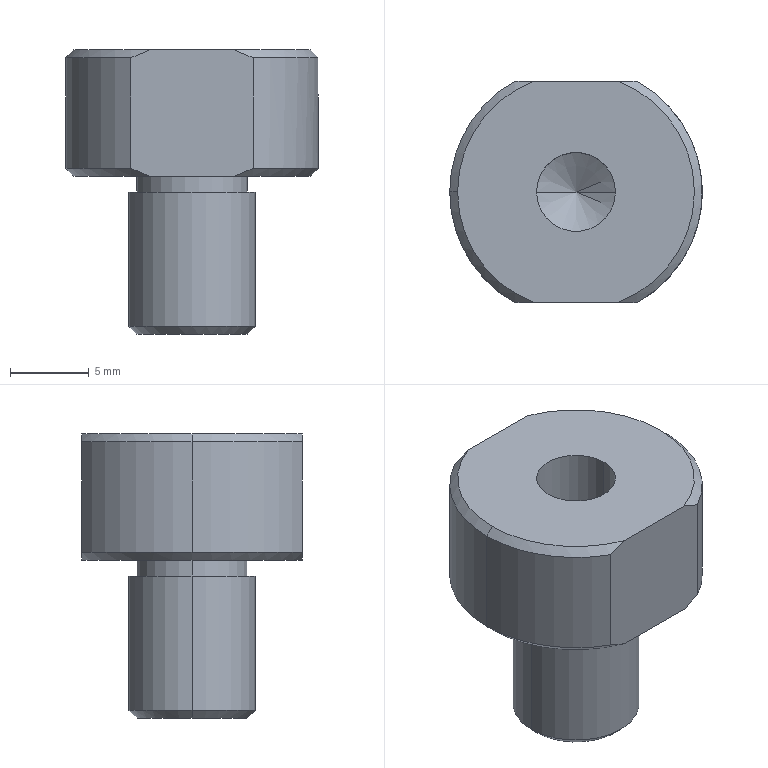Part | STEP file | 03-38 cylinder washer | 1 solid | 25 faces | box 16 x 14 x 18 mm | volume 1876 mm3 | cone 10 | cylinder 9 | plane 6 | commonest cylinder face diameters 16 x3 5 x2 7 x2 8 x2
STEP:
#1=CARTESIAN_POINT('',(-7.5,0.,8.));
#2=VERTEX_POINT('',#1);
#3=CARTESIAN_POINT('',(-2.693,-7.,8.));
#4=VERTEX_POINT('',#3);
#5=CARTESIAN_POINT('',(0.,0.,8.));
#6=DIRECTION('',(0.,0.,1.));
#7=DIRECTION('',(1.,0.,0.));
#8=AXIS2_PLACEMENT_3D('',#5,#6,#7);
#9=CIRCLE('',#8,7.5);
#10=EDGE_CURVE('',#2,#4,#9,.T.);
#11=ORIENTED_EDGE('',*,*,#10,.F.);
#12=CARTESIAN_POINT('',(-8.,0.,7.5));
#13=VERTEX_POINT('',#12);
#14=CARTESIAN_POINT('',(-7.5,0.,8.));
#15=DIRECTION('',(-0.7071,0.,-0.7071));
#16=VECTOR('',#15,1000.);
#17=LINE('',#14,#16);
#18=EDGE_CURVE('',#2,#13,#17,.T.);
#19=ORIENTED_EDGE('',*,*,#18,.T.);
#20=CARTESIAN_POINT('',(-3.873,-7.,7.5));
#21=VERTEX_POINT('',#20);
#22=CARTESIAN_POINT('',(0.,0.,7.5));
#23=DIRECTION('',(0.,0.,-1.));
#24=DIRECTION('',(1.,0.,0.));
#25=AXIS2_PLACEMENT_3D('',#22,#23,#24);
#26=CIRCLE('',#25,8.);
#27=EDGE_CURVE('',#21,#13,#26,.T.);
#28=ORIENTED_EDGE('',*,*,#27,.F.);
#29=CARTESIAN_POINT('',(-2.693,-7.,8.));
#30=CARTESIAN_POINT('',(-3.095,-7.,7.855));
#31=CARTESIAN_POINT('',(-3.488,-7.,7.686));
#32=CARTESIAN_POINT('',(-3.873,-7.,7.5));
#33=B_SPLINE_CURVE_WITH_KNOTS('',3,(#29,#30,#31,#32),.UNSPECIFIED.,.F.,.F.,(4,4),(0.,0.001282),.UNSPECIFIED.);
#34=EDGE_CURVE('',#4,#21,#33,.T.);
#35=ORIENTED_EDGE('',*,*,#34,.F.);
#36=EDGE_LOOP('',(#11,#19,#28,#35));
#37=FACE_OUTER_BOUND('',#36,.T.);
#38=CARTESIAN_POINT('',(0.,0.,8.));
#39=DIRECTION('',(0.,0.,-1.));
#40=DIRECTION('',(-1.,0.,0.));
#41=AXIS2_PLACEMENT_3D('',#38,#39,#40);
#42=CONICAL_SURFACE('',#41,7.5,0.7854);
#43=ADVANCED_FACE('',(#37),#42,.T.);
#44=CARTESIAN_POINT('',(7.5,0.,0.));
#45=VERTEX_POINT('',#44);
#46=CARTESIAN_POINT('',(2.693,-7.,0.));
#47=VERTEX_POINT('',#46);
#48=CARTESIAN_POINT('',(0.,0.,0.));
#49=DIRECTION('',(0.,0.,-1.));
#50=DIRECTION('',(1.,0.,0.));
#51=AXIS2_PLACEMENT_3D('',#48,#49,#50);
#52=CIRCLE('',#51,7.5);
#53=EDGE_CURVE('',#45,#47,#52,.T.);
#54=ORIENTED_EDGE('',*,*,#53,.F.);
#55=CARTESIAN_POINT('',(8.,0.,0.5));
#56=VERTEX_POINT('',#55);
#57=CARTESIAN_POINT('',(8.,0.,0.5));
#58=DIRECTION('',(0.7071,0.,0.7071));
#59=VECTOR('',#58,1000.);
#60=LINE('',#57,#59);
#61=EDGE_CURVE('',#45,#56,#60,.T.);
#62=ORIENTED_EDGE('',*,*,#61,.T.);
#63=CARTESIAN_POINT('',(3.873,-7.,0.5));
#64=VERTEX_POINT('',#63);
#65=CARTESIAN_POINT('',(0.,0.,0.5));
#66=DIRECTION('',(0.,0.,1.));
#67=DIRECTION('',(1.,0.,0.));
#68=AXIS2_PLACEMENT_3D('',#65,#66,#67);
#69=CIRCLE('',#68,8.);
#70=EDGE_CURVE('',#64,#56,#69,.T.);
#71=ORIENTED_EDGE('',*,*,#70,.F.);
#72=CARTESIAN_POINT('',(2.693,-7.,0.));
#73=CARTESIAN_POINT('',(3.095,-7.,0.1446));
#74=CARTESIAN_POINT('',(3.488,-7.,0.3136));
#75=CARTESIAN_POINT('',(3.873,-7.,0.5));
#76=B_SPLINE_CURVE_WITH_KNOTS('',3,(#72,#73,#74,#75),.UNSPECIFIED.,.F.,.F.,(4,4),(0.,0.001282),.UNSPECIFIED.);
#77=EDGE_CURVE('',#47,#64,#76,.T.);
#78=ORIENTED_EDGE('',*,*,#77,.F.);
#79=EDGE_LOOP('',(#54,#62,#71,#78));
#80=FACE_OUTER_BOUND('',#79,.T.);
#81=CARTESIAN_POINT('',(0.,0.,0.5));
#82=DIRECTION('',(0.,0.,1.));
#83=DIRECTION('',(1.,0.,0.));
#84=AXIS2_PLACEMENT_3D('',#81,#82,#83);
#85=CONICAL_SURFACE('',#84,8.,0.7854);
#86=ADVANCED_FACE('',(#80),#85,.T.);
#87=CARTESIAN_POINT('',(-2.5,0.,2.));
#88=VERTEX_POINT('',#87);
#89=CARTESIAN_POINT('',(2.5,0.,2.));
#90=VERTEX_POINT('',#89);
#91=CARTESIAN_POINT('',(0.,0.,2.));
#92=DIRECTION('',(0.,0.,1.));
#93=DIRECTION('',(1.,0.,0.));
#94=AXIS2_PLACEMENT_3D('',#91,#92,#93);
#95=CIRCLE('',#94,2.5);
#96=EDGE_CURVE('',#88,#90,#95,.T.);
#97=ORIENTED_EDGE('',*,*,#96,.F.);
#98=CARTESIAN_POINT('',(-2.5,0.,8.));
#99=VERTEX_POINT('',#98);
#100=CARTESIAN_POINT('',(-2.5,0.,8.));
#101=DIRECTION('',(0.,0.,1.));
#102=VECTOR('',#101,1000.);
#103=LINE('',#100,#102);
#104=EDGE_CURVE('',#88,#99,#103,.T.);
#105=ORIENTED_EDGE('',*,*,#104,.T.);
#106=CARTESIAN_POINT('',(2.5,0.,8.));
#107=VERTEX_POINT('',#106);
#108=CARTESIAN_POINT('',(0.,0.,8.));
#109=DIRECTION('',(0.,0.,1.));
#110=DIRECTION('',(1.,0.,0.));
#111=AXIS2_PLACEMENT_3D('',#108,#109,#110);
#112=CIRCLE('',#111,2.5);
#113=EDGE_CURVE('',#99,#107,#112,.T.);
#114=ORIENTED_EDGE('',*,*,#113,.T.);
#115=CARTESIAN_POINT('',(2.5,0.,8.));
#116=DIRECTION('',(0.,0.,1.));
#117=VECTOR('',#116,1000.);
#118=LINE('',#115,#117);
#119=EDGE_CURVE('',#90,#107,#118,.T.);
#120=ORIENTED_EDGE('',*,*,#119,.F.);
#121=EDGE_LOOP('',(#97,#105,#114,#120));
#122=FACE_OUTER_BOUND('',#121,.T.);
#123=CARTESIAN_POINT('',(0.,0.,8.));
#124=DIRECTION('',(0.,0.,1.));
#125=DIRECTION('',(1.,0.,0.));
#126=AXIS2_PLACEMENT_3D('',#123,#124,#125);
#127=CYLINDRICAL_SURFACE('',#126,2.5);
#128=ADVANCED_FACE('',(#122),#127,.F.);
#129=CARTESIAN_POINT('',(0.,0.,0.4978));
#130=VERTEX_POINT('',#129);
#131=CARTESIAN_POINT('',(2.5,0.,2.));
#132=DIRECTION('',(0.8572,0.,0.515));
#133=VECTOR('',#132,1000.);
#134=LINE('',#131,#133);
#135=EDGE_CURVE('',#130,#90,#134,.T.);
#136=ORIENTED_EDGE('',*,*,#135,.F.);
#137=CARTESIAN_POINT('',(-2.5,0.,2.));
#138=DIRECTION('',(-0.8572,0.,0.515));
#139=VECTOR('',#138,1000.);
#140=LINE('',#137,#139);
#141=EDGE_CURVE('',#130,#88,#140,.T.);
#142=ORIENTED_EDGE('',*,*,#141,.T.);
#143=ORIENTED_EDGE('',*,*,#96,.T.);
#144=EDGE_LOOP('',(#136,#142,#143));
#145=FACE_OUTER_BOUND('',#144,.T.);
#146=CARTESIAN_POINT('',(0.,0.,2.));
#147=DIRECTION('',(0.,0.,1.));
#148=DIRECTION('',(1.,0.,0.));
#149=AXIS2_PLACEMENT_3D('',#146,#147,#148);
#150=CONICAL_SURFACE('',#149,2.5,1.03);
#151=ADVANCED_FACE('',(#145),#150,.F.);
#152=CARTESIAN_POINT('',(-3.5,0.,-10.));
#153=VERTEX_POINT('',#152);
#154=CARTESIAN_POINT('',(3.5,0.,-10.));
#155=VERTEX_POINT('',#154);
#156=CARTESIAN_POINT('',(0.,0.,-10.));
#157=DIRECTION('',(0.,0.,-1.));
#158=DIRECTION('',(-1.,0.,0.));
#159=AXIS2_PLACEMENT_3D('',#156,#157,#158);
#160=CIRCLE('',#159,3.5);
#161=EDGE_CURVE('',#153,#155,#160,.T.);
#162=ORIENTED_EDGE('',*,*,#161,.F.);
#163=CARTESIAN_POINT('',(-4.,0.,-9.5));
#164=VERTEX_POINT('',#163);
#165=CARTESIAN_POINT('',(-3.5,0.,-10.));
#166=DIRECTION('',(-0.7071,0.,0.7071));
#167=VECTOR('',#166,1000.);
#168=LINE('',#165,#167);
#169=EDGE_CURVE('',#153,#164,#168,.T.);
#170=ORIENTED_EDGE('',*,*,#169,.T.);
#171=CARTESIAN_POINT('',(4.,0.,-9.5));
#172=VERTEX_POINT('',#171);
#173=CARTESIAN_POINT('',(0.,0.,-9.5));
#174=DIRECTION('',(0.,0.,1.));
#175=DIRECTION('',(-1.,0.,0.));
#176=AXIS2_PLACEMENT_3D('',#173,#174,#175);
#177=CIRCLE('',#176,4.);
#178=EDGE_CURVE('',#172,#164,#177,.T.);
#179=ORIENTED_EDGE('',*,*,#178,.F.);
#180=CARTESIAN_POINT('',(3.5,0.,-10.));
#181=DIRECTION('',(0.7071,0.,0.7071));
#182=VECTOR('',#181,1000.);
#183=LINE('',#180,#182);
#184=EDGE_CURVE('',#155,#172,#183,.T.);
#185=ORIENTED_EDGE('',*,*,#184,.F.);
#186=EDGE_LOOP('',(#162,#170,#179,#185));
#187=FACE_OUTER_BOUND('',#186,.T.);
#188=CARTESIAN_POINT('',(0.,0.,-10.));
#189=DIRECTION('',(0.,0.,1.));
#190=DIRECTION('',(1.,0.,0.));
#191=AXIS2_PLACEMENT_3D('',#188,#189,#190);
#192=CONICAL_SURFACE('',#191,3.5,0.7854);
#193=ADVANCED_FACE('',(#187),#192,.T.);
#194=ORIENTED_EDGE('',*,*,#178,.T.);
#195=CARTESIAN_POINT('',(-4.,0.,-1.));
#196=VERTEX_POINT('',#195);
#197=CARTESIAN_POINT('',(-4.,0.,-10.));
#198=DIRECTION('',(0.,0.,1.));
#199=VECTOR('',#198,1000.);
#200=LINE('',#197,#199);
#201=EDGE_CURVE('',#164,#196,#200,.T.);
#202=ORIENTED_EDGE('',*,*,#201,.T.);
#203=CARTESIAN_POINT('',(4.,0.,-1.));
#204=VERTEX_POINT('',#203);
#205=CARTESIAN_POINT('',(0.,0.,-1.));
#206=DIRECTION('',(0.,0.,-1.));
#207=DIRECTION('',(-1.,0.,0.));
#208=AXIS2_PLACEMENT_3D('',#205,#206,#207);
#209=CIRCLE('',#208,4.);
#210=EDGE_CURVE('',#196,#204,#209,.T.);
#211=ORIENTED_EDGE('',*,*,#210,.T.);
#212=CARTESIAN_POINT('',(4.,0.,-10.));
#213=DIRECTION('',(0.,0.,1.));
#214=VECTOR('',#213,1000.);
#215=LINE('',#212,#214);
#216=EDGE_CURVE('',#172,#204,#215,.T.);
#217=ORIENTED_EDGE('',*,*,#216,.F.);
#218=EDGE_LOOP('',(#194,#202,#211,#217));
#219=FACE_OUTER_BOUND('',#218,.T.);
#220=CARTESIAN_POINT('',(0.,0.,-10.));
#221=DIRECTION('',(0.,0.,1.));
#222=DIRECTION('',(1.,0.,0.));
#223=AXIS2_PLACEMENT_3D('',#220,#221,#222);
#224=CYLINDRICAL_SURFACE('',#223,4.);
#225=ADVANCED_FACE('',(#219),#224,.T.);
#226=CARTESIAN_POINT('',(-3.5,0.,-1.));
#227=VERTEX_POINT('',#226);
#228=CARTESIAN_POINT('',(3.5,0.,-1.));
#229=VERTEX_POINT('',#228);
#230=CARTESIAN_POINT('',(0.,0.,-1.));
#231=DIRECTION('',(0.,0.,-1.));
#232=DIRECTION('',(-1.,0.,0.));
#233=AXIS2_PLACEMENT_3D('',#230,#231,#232);
#234=CIRCLE('',#233,3.5);
#235=EDGE_CURVE('',#227,#229,#234,.T.);
#236=ORIENTED_EDGE('',*,*,#235,.F.);
#237=CARTESIAN_POINT('',(-3.5,0.,0.));
#238=VERTEX_POINT('',#237);
#239=CARTESIAN_POINT('',(-3.5,0.,-1.));
#240=DIRECTION('',(0.,0.,1.));
#241=VECTOR('',#240,1000.);
#242=LINE('',#239,#241);
#243=EDGE_CURVE('',#227,#238,#242,.T.);
#244=ORIENTED_EDGE('',*,*,#243,.T.);
#245=CARTESIAN_POINT('',(3.5,0.,0.));
#246=VERTEX_POINT('',#245);
#247=CARTESIAN_POINT('',(0.,0.,0.));
#248=DIRECTION('',(0.,0.,-1.));
#249=DIRECTION('',(1.,0.,0.));
#250=AXIS2_PLACEMENT_3D('',#247,#248,#249);
#251=CIRCLE('',#250,3.5);
#252=EDGE_CURVE('',#238,#246,#251,.T.);
#253=ORIENTED_EDGE('',*,*,#252,.T.);
#254=CARTESIAN_POINT('',(3.5,0.,-1.));
#255=DIRECTION('',(0.,0.,1.));
#256=VECTOR('',#255,1000.);
#257=LINE('',#254,#256);
#258=EDGE_CURVE('',#229,#246,#257,.T.);
#259=ORIENTED_EDGE('',*,*,#258,.F.);
#260=EDGE_LOOP('',(#236,#244,#253,#259));
#261=FACE_OUTER_BOUND('',#260,.T.);
#262=CARTESIAN_POINT('',(0.,0.,-1.));
#263=DIRECTION('',(0.,0.,1.));
#264=DIRECTION('',(1.,0.,0.));
#265=AXIS2_PLACEMENT_3D('',#262,#263,#264);
#266=CYLINDRICAL_SURFACE('',#265,3.5);
#267=ADVANCED_FACE('',(#261),#266,.T.);
#268=ORIENTED_EDGE('',*,*,#27,.T.);
#269=CARTESIAN_POINT('',(-8.,0.,0.5));
#270=VERTEX_POINT('',#269);
#271=CARTESIAN_POINT('',(-8.,0.,8.));
#272=DIRECTION('',(0.,0.,-1.));
#273=VECTOR('',#272,1000.);
#274=LINE('',#271,#273);
#275=EDGE_CURVE('',#13,#270,#274,.T.);
#276=ORIENTED_EDGE('',*,*,#275,.T.);
#277=CARTESIAN_POINT('',(-3.873,-7.,0.5));
#278=VERTEX_POINT('',#277);
#279=CARTESIAN_POINT('',(0.,0.,0.5));
#280=DIRECTION('',(0.,0.,1.));
#281=DIRECTION('',(1.,0.,0.));
#282=AXIS2_PLACEMENT_3D('',#279,#280,#281);
#283=CIRCLE('',#282,8.);
#284=EDGE_CURVE('',#270,#278,#283,.T.);
#285=ORIENTED_EDGE('',*,*,#284,.T.);
#286=CARTESIAN_POINT('',(-3.873,-7.,8.));
#287=DIRECTION('',(0.,0.,1.));
#288=VECTOR('',#287,1000.);
#289=LINE('',#286,#288);
#290=EDGE_CURVE('',#278,#21,#289,.T.);
#291=ORIENTED_EDGE('',*,*,#290,.T.);
#292=EDGE_LOOP('',(#268,#276,#285,#291));
#293=FACE_OUTER_BOUND('',#292,.T.);
#294=CARTESIAN_POINT('',(0.,0.,8.));
#295=DIRECTION('',(0.,0.,-1.));
#296=DIRECTION('',(-1.,0.,0.));
#297=AXIS2_PLACEMENT_3D('',#294,#295,#296);
#298=CYLINDRICAL_SURFACE('',#297,8.);
#299=ADVANCED_FACE('',(#293),#298,.T.);
#300=CARTESIAN_POINT('',(3.873,-7.,7.5));
#301=VERTEX_POINT('',#300);
#302=CARTESIAN_POINT('',(3.873,-7.,8.));
#303=DIRECTION('',(0.,0.,-1.));
#304=VECTOR('',#303,1000.);
#305=LINE('',#302,#304);
#306=EDGE_CURVE('',#301,#64,#305,.T.);
#307=ORIENTED_EDGE('',*,*,#306,.T.);
#308=ORIENTED_EDGE('',*,*,#70,.T.);
#309=CARTESIAN_POINT('',(3.873,7.,0.5));
#310=VERTEX_POINT('',#309);
#311=CARTESIAN_POINT('',(0.,0.,0.5));
#312=DIRECTION('',(0.,0.,1.));
#313=DIRECTION('',(1.,0.,0.));
#314=AXIS2_PLACEMENT_3D('',#311,#312,#313);
#315=CIRCLE('',#314,8.);
#316=EDGE_CURVE('',#56,#310,#315,.T.);
#317=ORIENTED_EDGE('',*,*,#316,.T.);
#318=CARTESIAN_POINT('',(3.873,7.,7.5));
#319=VERTEX_POINT('',#318);
#320=CARTESIAN_POINT('',(3.873,7.,8.));
#321=DIRECTION('',(0.,0.,1.));
#322=VECTOR('',#321,1000.);
#323=LINE('',#320,#322);
#324=EDGE_CURVE('',#310,#319,#323,.T.);
#325=ORIENTED_EDGE('',*,*,#324,.T.);
#326=CARTESIAN_POINT('',(0.,0.,7.5));
#327=DIRECTION('',(0.,0.,-1.));
#328=DIRECTION('',(1.,0.,0.));
#329=AXIS2_PLACEMENT_3D('',#326,#327,#328);
#330=CIRCLE('',#329,8.);
#331=EDGE_CURVE('',#319,#301,#330,.T.);
#332=ORIENTED_EDGE('',*,*,#331,.T.);
#333=EDGE_LOOP('',(#307,#308,#317,#325,#332));
#334=FACE_OUTER_BOUND('',#333,.T.);
#335=CARTESIAN_POINT('',(0.,0.,8.));
#336=DIRECTION('',(0.,0.,-1.));
#337=DIRECTION('',(-1.,0.,0.));
#338=AXIS2_PLACEMENT_3D('',#335,#336,#337);
#339=CYLINDRICAL_SURFACE('',#338,8.);
#340=ADVANCED_FACE('',(#334),#339,.T.);
#341=CARTESIAN_POINT('',(-2.693,7.,0.));
#342=VERTEX_POINT('',#341);
#343=CARTESIAN_POINT('',(2.693,7.,0.));
#344=VERTEX_POINT('',#343);
#345=CARTESIAN_POINT('',(-4.544,7.,0.));
#346=DIRECTION('',(1.,0.,0.));
#347=VECTOR('',#346,1000.);
#348=LINE('',#345,#347);
#349=EDGE_CURVE('',#342,#344,#348,.T.);
#350=ORIENTED_EDGE('',*,*,#349,.T.);
#351=CARTESIAN_POINT('',(0.,0.,0.));
#352=DIRECTION('',(0.,0.,-1.));
#353=DIRECTION('',(1.,0.,0.));
#354=AXIS2_PLACEMENT_3D('',#351,#352,#353);
#355=CIRCLE('',#354,7.5);
#356=EDGE_CURVE('',#344,#45,#355,.T.);
#357=ORIENTED_EDGE('',*,*,#356,.T.);
#358=ORIENTED_EDGE('',*,*,#53,.T.);
#359=CARTESIAN_POINT('',(-2.693,-7.,0.));
#360=VERTEX_POINT('',#359);
#361=CARTESIAN_POINT('',(-4.544,-7.,0.));
#362=DIRECTION('',(-1.,0.,0.));
#363=VECTOR('',#362,1000.);
#364=LINE('',#361,#363);
#365=EDGE_CURVE('',#47,#360,#364,.T.);
#366=ORIENTED_EDGE('',*,*,#365,.T.);
#367=CARTESIAN_POINT('',(0.,0.,0.));
#368=DIRECTION('',(0.,0.,-1.));
#369=DIRECTION('',(1.,0.,0.));
#370=AXIS2_PLACEMENT_3D('',#367,#368,#369);
#371=CIRCLE('',#370,7.5);
#372=EDGE_CURVE('',#360,#342,#371,.T.);
#373=ORIENTED_EDGE('',*,*,#372,.T.);
#374=EDGE_LOOP('',(#350,#357,#358,#366,#373));
#375=FACE_OUTER_BOUND('',#374,.T.);
#376=CARTESIAN_POINT('',(0.,0.,0.));
#377=DIRECTION('',(0.,0.,-1.));
#378=DIRECTION('',(1.,0.,0.));
#379=AXIS2_PLACEMENT_3D('',#376,#377,#378);
#380=CIRCLE('',#379,3.5);
#381=EDGE_CURVE('',#246,#238,#380,.T.);
#382=ORIENTED_EDGE('',*,*,#381,.F.);
#383=ORIENTED_EDGE('',*,*,#252,.F.);
#384=EDGE_LOOP('',(#382,#383));
#385=FACE_BOUND('',#384,.T.);
#386=CARTESIAN_POINT('',(0.,0.,0.));
#387=DIRECTION('',(0.,0.,1.));
#388=DIRECTION('',(1.,0.,0.));
#389=AXIS2_PLACEMENT_3D('',#386,#387,#388);
#390=PLANE('',#389);
#391=ADVANCED_FACE('',(#375,#385),#390,.F.);
#392=ORIENTED_EDGE('',*,*,#275,.F.);
#393=CARTESIAN_POINT('',(-3.873,7.,7.5));
#394=VERTEX_POINT('',#393);
#395=CARTESIAN_POINT('',(0.,0.,7.5));
#396=DIRECTION('',(0.,0.,-1.));
#397=DIRECTION('',(1.,0.,0.));
#398=AXIS2_PLACEMENT_3D('',#395,#396,#397);
#399=CIRCLE('',#398,8.);
#400=EDGE_CURVE('',#13,#394,#399,.T.);
#401=ORIENTED_EDGE('',*,*,#400,.T.);
#402=CARTESIAN_POINT('',(-3.873,7.,0.5));
#403=VERTEX_POINT('',#402);
#404=CARTESIAN_POINT('',(-3.873,7.,8.));
#405=DIRECTION('',(0.,0.,-1.));
#406=VECTOR('',#405,1000.);
#407=LINE('',#404,#406);
#408=EDGE_CURVE('',#394,#403,#407,.T.);
#409=ORIENTED_EDGE('',*,*,#408,.T.);
#410=CARTESIAN_POINT('',(0.,0.,0.5));
#411=DIRECTION('',(0.,0.,1.));
#412=DIRECTION('',(1.,0.,0.));
#413=AXIS2_PLACEMENT_3D('',#410,#411,#412);
#414=CIRCLE('',#413,8.);
#415=EDGE_CURVE('',#403,#270,#414,.T.);
#416=ORIENTED_EDGE('',*,*,#415,.T.);
#417=EDGE_LOOP('',(#392,#401,#409,#416));
#418=FACE_OUTER_BOUND('',#417,.T.);
#419=CARTESIAN_POINT('',(0.,0.,8.));
#420=DIRECTION('',(0.,0.,-1.));
#421=DIRECTION('',(-1.,0.,0.));
#422=AXIS2_PLACEMENT_3D('',#419,#420,#421);
#423=CYLINDRICAL_SURFACE('',#422,8.);
#424=ADVANCED_FACE('',(#418),#423,.T.);
#425=CARTESIAN_POINT('',(0.,0.,8.));
#426=DIRECTION('',(0.,0.,1.));
#427=DIRECTION('',(1.,0.,0.));
#428=AXIS2_PLACEMENT_3D('',#425,#426,#427);
#429=CIRCLE('',#428,2.5);
#430=EDGE_CURVE('',#107,#99,#429,.T.);
#431=ORIENTED_EDGE('',*,*,#430,.F.);
#432=ORIENTED_EDGE('',*,*,#113,.F.);
#433=EDGE_LOOP('',(#431,#432));
#434=FACE_BOUND('',#433,.T.);
#435=CARTESIAN_POINT('',(2.693,-7.,8.));
#436=VERTEX_POINT('',#435);
#437=CARTESIAN_POINT('',(0.,-7.,8.));
#438=DIRECTION('',(-1.,0.,0.));
#439=VECTOR('',#438,1000.);
#440=LINE('',#437,#439);
#441=EDGE_CURVE('',#436,#4,#440,.T.);
#442=ORIENTED_EDGE('',*,*,#441,.F.);
#443=CARTESIAN_POINT('',(2.693,7.,8.));
#444=VERTEX_POINT('',#443);
#445=CARTESIAN_POINT('',(0.,0.,8.));
#446=DIRECTION('',(0.,0.,1.));
#447=DIRECTION('',(1.,0.,0.));
#448=AXIS2_PLACEMENT_3D('',#445,#446,#447);
#449=CIRCLE('',#448,7.5);
#450=EDGE_CURVE('',#436,#444,#449,.T.);
#451=ORIENTED_EDGE('',*,*,#450,.T.);
#452=CARTESIAN_POINT('',(-2.693,7.,8.));
#453=VERTEX_POINT('',#452);
#454=CARTESIAN_POINT('',(0.,7.,8.));
#455=DIRECTION('',(1.,0.,0.));
#456=VECTOR('',#455,1000.);
#457=LINE('',#454,#456);
#458=EDGE_CURVE('',#453,#444,#457,.T.);
#459=ORIENTED_EDGE('',*,*,#458,.F.);
#460=CARTESIAN_POINT('',(0.,0.,8.));
#461=DIRECTION('',(0.,0.,1.));
#462=DIRECTION('',(1.,0.,0.));
#463=AXIS2_PLACEMENT_3D('',#460,#461,#462);
#464=CIRCLE('',#463,7.5);
#465=EDGE_CURVE('',#453,#2,#464,.T.);
#466=ORIENTED_EDGE('',*,*,#465,.T.);
#467=ORIENTED_EDGE('',*,*,#10,.T.);
#468=EDGE_LOOP('',(#442,#451,#459,#466,#467));
#469=FACE_OUTER_BOUND('',#468,.T.);
#470=CARTESIAN_POINT('',(0.,0.,8.));
#471=DIRECTION('',(0.,0.,1.));
#472=DIRECTION('',(1.,0.,0.));
#473=AXIS2_PLACEMENT_3D('',#470,#471,#472);
#474=PLANE('',#473);
#475=ADVANCED_FACE('',(#434,#469),#474,.T.);
#476=ORIENTED_EDGE('',*,*,#243,.F.);
#477=CARTESIAN_POINT('',(0.,0.,-1.));
#478=DIRECTION('',(0.,0.,-1.));
#479=DIRECTION('',(-1.,0.,0.));
#480=AXIS2_PLACEMENT_3D('',#477,#478,#479);
#481=CIRCLE('',#480,3.5);
#482=EDGE_CURVE('',#229,#227,#481,.T.);
#483=ORIENTED_EDGE('',*,*,#482,.F.);
#484=ORIENTED_EDGE('',*,*,#258,.T.);
#485=ORIENTED_EDGE('',*,*,#381,.T.);
#486=EDGE_LOOP('',(#476,#483,#484,#485));
#487=FACE_OUTER_BOUND('',#486,.T.);
#488=CARTESIAN_POINT('',(0.,0.,-1.));
#489=DIRECTION('',(0.,0.,1.));
#490=DIRECTION('',(1.,0.,0.));
#491=AXIS2_PLACEMENT_3D('',#488,#489,#490);
#492=CYLINDRICAL_SURFACE('',#491,3.5);
#493=ADVANCED_FACE('',(#487),#492,.T.);
#494=CARTESIAN_POINT('',(0.,0.,-1.));
#495=DIRECTION('',(0.,0.,-1.));
#496=DIRECTION('',(-1.,0.,0.));
#497=AXIS2_PLACEMENT_3D('',#494,#495,#496);
#498=CIRCLE('',#497,4.);
#499=EDGE_CURVE('',#204,#196,#498,.T.);
#500=ORIENTED_EDGE('',*,*,#499,.F.);
#501=ORIENTED_EDGE('',*,*,#210,.F.);
#502=EDGE_LOOP('',(#500,#501));
#503=FACE_OUTER_BOUND('',#502,.T.);
#504=ORIENTED_EDGE('',*,*,#482,.T.);
#505=ORIENTED_EDGE('',*,*,#235,.T.);
#506=EDGE_LOOP('',(#504,#505));
#507=FACE_BOUND('',#506,.T.);
#508=CARTESIAN_POINT('',(0.,0.,-1.));
#509=DIRECTION('',(0.,0.,-1.));
#510=DIRECTION('',(-1.,0.,0.));
#511=AXIS2_PLACEMENT_3D('',#508,#509,#510);
#512=PLANE('',#511);
#513=ADVANCED_FACE('',(#503,#507),#512,.F.);
#514=ORIENTED_EDGE('',*,*,#201,.F.);
#515=CARTESIAN_POINT('',(0.,0.,-9.5));
#516=DIRECTION('',(0.,0.,1.));
#517=DIRECTION('',(-1.,0.,0.));
#518=AXIS2_PLACEMENT_3D('',#515,#516,#517);
#519=CIRCLE('',#518,4.);
#520=EDGE_CURVE('',#164,#172,#519,.T.);
#521=ORIENTED_EDGE('',*,*,#520,.T.);
#522=ORIENTED_EDGE('',*,*,#216,.T.);
#523=ORIENTED_EDGE('',*,*,#499,.T.);
#524=EDGE_LOOP('',(#514,#521,#522,#523));
#525=FACE_OUTER_BOUND('',#524,.T.);
#526=CARTESIAN_POINT('',(0.,0.,-10.));
#527=DIRECTION('',(0.,0.,1.));
#528=DIRECTION('',(1.,0.,0.));
#529=AXIS2_PLACEMENT_3D('',#526,#527,#528);
#530=CYLINDRICAL_SURFACE('',#529,4.);
#531=ADVANCED_FACE('',(#525),#530,.T.);
#532=CARTESIAN_POINT('',(0.,0.,-10.));
#533=DIRECTION('',(0.,0.,-1.));
#534=DIRECTION('',(-1.,0.,0.));
#535=AXIS2_PLACEMENT_3D('',#532,#533,#534);
#536=CIRCLE('',#535,3.5);
#537=EDGE_CURVE('',#155,#153,#536,.T.);
#538=ORIENTED_EDGE('',*,*,#537,.T.);
#539=ORIENTED_EDGE('',*,*,#161,.T.);
#540=EDGE_LOOP('',(#538,#539));
#541=FACE_OUTER_BOUND('',#540,.T.);
#542=CARTESIAN_POINT('',(0.,0.,-10.));
#543=DIRECTION('',(0.,0.,-1.));
#544=DIRECTION('',(-1.,0.,0.));
#545=AXIS2_PLACEMENT_3D('',#542,#543,#544);
#546=PLANE('',#545);
#547=ADVANCED_FACE('',(#541),#546,.T.);
#548=ORIENTED_EDGE('',*,*,#169,.F.);
#549=ORIENTED_EDGE('',*,*,#537,.F.);
#550=ORIENTED_EDGE('',*,*,#184,.T.);
#551=ORIENTED_EDGE('',*,*,#520,.F.);
#552=EDGE_LOOP('',(#548,#549,#550,#551));
#553=FACE_OUTER_BOUND('',#552,.T.);
#554=CARTESIAN_POINT('',(0.,0.,-10.));
#555=DIRECTION('',(0.,0.,1.));
#556=DIRECTION('',(1.,0.,0.));
#557=AXIS2_PLACEMENT_3D('',#554,#555,#556);
#558=CONICAL_SURFACE('',#557,3.5,0.7854);
#559=ADVANCED_FACE('',(#553),#558,.T.);
#560=ORIENTED_EDGE('',*,*,#324,.F.);
#561=CARTESIAN_POINT('',(3.873,7.,0.5));
#562=CARTESIAN_POINT('',(3.488,7.,0.3136));
#563=CARTESIAN_POINT('',(3.095,7.,0.1446));
#564=CARTESIAN_POINT('',(2.693,7.,0.));
#565=B_SPLINE_CURVE_WITH_KNOTS('',3,(#561,#562,#563,#564),.UNSPECIFIED.,.F.,.F.,(4,4),(0.,0.001282),.UNSPECIFIED.);
#566=EDGE_CURVE('',#310,#344,#565,.T.);
#567=ORIENTED_EDGE('',*,*,#566,.T.);
#568=ORIENTED_EDGE('',*,*,#349,.F.);
#569=CARTESIAN_POINT('',(-2.693,7.,0.));
#570=CARTESIAN_POINT('',(-3.095,7.,0.1446));
#571=CARTESIAN_POINT('',(-3.488,7.,0.3136));
#572=CARTESIAN_POINT('',(-3.873,7.,0.5));
#573=B_SPLINE_CURVE_WITH_KNOTS('',3,(#569,#570,#571,#572),.UNSPECIFIED.,.F.,.F.,(4,4),(0.,0.001282),.UNSPECIFIED.);
#574=EDGE_CURVE('',#342,#403,#573,.T.);
#575=ORIENTED_EDGE('',*,*,#574,.T.);
#576=ORIENTED_EDGE('',*,*,#408,.F.);
#577=CARTESIAN_POINT('',(-3.873,7.,7.5));
#578=CARTESIAN_POINT('',(-3.488,7.,7.686));
#579=CARTESIAN_POINT('',(-3.095,7.,7.855));
#580=CARTESIAN_POINT('',(-2.693,7.,8.));
#581=B_SPLINE_CURVE_WITH_KNOTS('',3,(#577,#578,#579,#580),.UNSPECIFIED.,.F.,.F.,(4,4),(0.,0.001282),.UNSPECIFIED.);
#582=EDGE_CURVE('',#394,#453,#581,.T.);
#583=ORIENTED_EDGE('',*,*,#582,.T.);
#584=ORIENTED_EDGE('',*,*,#458,.T.);
#585=CARTESIAN_POINT('',(2.693,7.,8.));
#586=CARTESIAN_POINT('',(3.095,7.,7.855));
#587=CARTESIAN_POINT('',(3.488,7.,7.686));
#588=CARTESIAN_POINT('',(3.873,7.,7.5));
#589=B_SPLINE_CURVE_WITH_KNOTS('',3,(#585,#586,#587,#588),.UNSPECIFIED.,.F.,.F.,(4,4),(0.,0.001282),.UNSPECIFIED.);
#590=EDGE_CURVE('',#444,#319,#589,.T.);
#591=ORIENTED_EDGE('',*,*,#590,.T.);
#592=EDGE_LOOP('',(#560,#567,#568,#575,#576,#583,#584,#591));
#593=FACE_OUTER_BOUND('',#592,.T.);
#594=CARTESIAN_POINT('',(-4.544,7.,0.));
#595=DIRECTION('',(0.,-1.,0.));
#596=DIRECTION('',(0.,0.,-1.));
#597=AXIS2_PLACEMENT_3D('',#594,#595,#596);
#598=PLANE('',#597);
#599=ADVANCED_FACE('',(#593),#598,.F.);
#600=ORIENTED_EDGE('',*,*,#365,.F.);
#601=ORIENTED_EDGE('',*,*,#77,.T.);
#602=ORIENTED_EDGE('',*,*,#306,.F.);
#603=CARTESIAN_POINT('',(3.873,-7.,7.5));
#604=CARTESIAN_POINT('',(3.488,-7.,7.686));
#605=CARTESIAN_POINT('',(3.095,-7.,7.855));
#606=CARTESIAN_POINT('',(2.693,-7.,8.));
#607=B_SPLINE_CURVE_WITH_KNOTS('',3,(#603,#604,#605,#606),.UNSPECIFIED.,.F.,.F.,(4,4),(0.,0.001282),.UNSPECIFIED.);
#608=EDGE_CURVE('',#301,#436,#607,.T.);
#609=ORIENTED_EDGE('',*,*,#608,.T.);
#610=ORIENTED_EDGE('',*,*,#441,.T.);
#611=ORIENTED_EDGE('',*,*,#34,.T.);
#612=ORIENTED_EDGE('',*,*,#290,.F.);
#613=CARTESIAN_POINT('',(-3.873,-7.,0.5));
#614=CARTESIAN_POINT('',(-3.488,-7.,0.3136));
#615=CARTESIAN_POINT('',(-3.095,-7.,0.1446));
#616=CARTESIAN_POINT('',(-2.693,-7.,0.));
#617=B_SPLINE_CURVE_WITH_KNOTS('',3,(#613,#614,#615,#616),.UNSPECIFIED.,.F.,.F.,(4,4),(0.,0.001282),.UNSPECIFIED.);
#618=EDGE_CURVE('',#278,#360,#617,.T.);
#619=ORIENTED_EDGE('',*,*,#618,.T.);
#620=EDGE_LOOP('',(#600,#601,#602,#609,#610,#611,#612,#619));
#621=FACE_OUTER_BOUND('',#620,.T.);
#622=CARTESIAN_POINT('',(-4.544,-7.,0.));
#623=DIRECTION('',(0.,1.,0.));
#624=DIRECTION('',(0.,0.,1.));
#625=AXIS2_PLACEMENT_3D('',#622,#623,#624);
#626=PLANE('',#625);
#627=ADVANCED_FACE('',(#621),#626,.F.);
#628=ORIENTED_EDGE('',*,*,#141,.F.);
#629=ORIENTED_EDGE('',*,*,#135,.T.);
#630=CARTESIAN_POINT('',(0.,0.,2.));
#631=DIRECTION('',(0.,0.,1.));
#632=DIRECTION('',(1.,0.,0.));
#633=AXIS2_PLACEMENT_3D('',#630,#631,#632);
#634=CIRCLE('',#633,2.5);
#635=EDGE_CURVE('',#90,#88,#634,.T.);
#636=ORIENTED_EDGE('',*,*,#635,.T.);
#637=EDGE_LOOP('',(#628,#629,#636));
#638=FACE_OUTER_BOUND('',#637,.T.);
#639=CARTESIAN_POINT('',(0.,0.,2.));
#640=DIRECTION('',(0.,0.,1.));
#641=DIRECTION('',(1.,0.,0.));
#642=AXIS2_PLACEMENT_3D('',#639,#640,#641);
#643=CONICAL_SURFACE('',#642,2.5,1.03);
#644=ADVANCED_FACE('',(#638),#643,.F.);
#645=ORIENTED_EDGE('',*,*,#104,.F.);
#646=ORIENTED_EDGE('',*,*,#635,.F.);
#647=ORIENTED_EDGE('',*,*,#119,.T.);
#648=ORIENTED_EDGE('',*,*,#430,.T.);
#649=EDGE_LOOP('',(#645,#646,#647,#648));
#650=FACE_OUTER_BOUND('',#649,.T.);
#651=CARTESIAN_POINT('',(0.,0.,8.));
#652=DIRECTION('',(0.,0.,1.));
#653=DIRECTION('',(1.,0.,0.));
#654=AXIS2_PLACEMENT_3D('',#651,#652,#653);
#655=CYLINDRICAL_SURFACE('',#654,2.5);
#656=ADVANCED_FACE('',(#650),#655,.F.);
#657=ORIENTED_EDGE('',*,*,#61,.F.);
#658=ORIENTED_EDGE('',*,*,#356,.F.);
#659=ORIENTED_EDGE('',*,*,#566,.F.);
#660=ORIENTED_EDGE('',*,*,#316,.F.);
#661=EDGE_LOOP('',(#657,#658,#659,#660));
#662=FACE_OUTER_BOUND('',#661,.T.);
#663=CARTESIAN_POINT('',(0.,0.,0.5));
#664=DIRECTION('',(0.,0.,1.));
#665=DIRECTION('',(1.,0.,0.));
#666=AXIS2_PLACEMENT_3D('',#663,#664,#665);
#667=CONICAL_SURFACE('',#666,8.,0.7854);
#668=ADVANCED_FACE('',(#662),#667,.T.);
#669=ORIENTED_EDGE('',*,*,#608,.F.);
#670=ORIENTED_EDGE('',*,*,#331,.F.);
#671=ORIENTED_EDGE('',*,*,#590,.F.);
#672=ORIENTED_EDGE('',*,*,#450,.F.);
#673=EDGE_LOOP('',(#669,#670,#671,#672));
#674=FACE_OUTER_BOUND('',#673,.T.);
#675=CARTESIAN_POINT('',(0.,0.,8.));
#676=DIRECTION('',(0.,0.,-1.));
#677=DIRECTION('',(-1.,0.,0.));
#678=AXIS2_PLACEMENT_3D('',#675,#676,#677);
#679=CONICAL_SURFACE('',#678,7.5,0.7854);
#680=ADVANCED_FACE('',(#674),#679,.T.);
#681=ORIENTED_EDGE('',*,*,#574,.F.);
#682=ORIENTED_EDGE('',*,*,#372,.F.);
#683=ORIENTED_EDGE('',*,*,#618,.F.);
#684=ORIENTED_EDGE('',*,*,#284,.F.);
#685=ORIENTED_EDGE('',*,*,#415,.F.);
#686=EDGE_LOOP('',(#681,#682,#683,#684,#685));
#687=FACE_OUTER_BOUND('',#686,.T.);
#688=CARTESIAN_POINT('',(0.,0.,0.5));
#689=DIRECTION('',(0.,0.,1.));
#690=DIRECTION('',(1.,0.,0.));
#691=AXIS2_PLACEMENT_3D('',#688,#689,#690);
#692=CONICAL_SURFACE('',#691,8.,0.7854);
#693=ADVANCED_FACE('',(#687),#692,.T.);
#694=ORIENTED_EDGE('',*,*,#18,.F.);
#695=ORIENTED_EDGE('',*,*,#465,.F.);
#696=ORIENTED_EDGE('',*,*,#582,.F.);
#697=ORIENTED_EDGE('',*,*,#400,.F.);
#698=EDGE_LOOP('',(#694,#695,#696,#697));
#699=FACE_OUTER_BOUND('',#698,.T.);
#700=CARTESIAN_POINT('',(0.,0.,8.));
#701=DIRECTION('',(0.,0.,-1.));
#702=DIRECTION('',(-1.,0.,0.));
#703=AXIS2_PLACEMENT_3D('',#700,#701,#702);
#704=CONICAL_SURFACE('',#703,7.5,0.7854);
#705=ADVANCED_FACE('',(#699),#704,.T.);
#706=CLOSED_SHELL('',(#43,#86,#128,#151,#193,#225,#267,#299,#340,#391,#424,#475,#493,#513,#531,#547,#559,#599,#627,#644,#656,#668,#680,#693,#705));
#707=MANIFOLD_SOLID_BREP('',#706);
#708=CARTESIAN_POINT('',(0.,0.,0.));
#709=DIRECTION('',(0.,0.,1.));
#710=DIRECTION('',(1.,0.,0.));
#711=AXIS2_PLACEMENT_3D('',#708,#709,#710);
#712=(LENGTH_UNIT()NAMED_UNIT(*)SI_UNIT(.MILLI.,.METRE.));
#713=UNCERTAINTY_MEASURE_WITH_UNIT(LENGTH_MEASURE(0.00001),#712,'','');
#714=(NAMED_UNIT(*)PLANE_ANGLE_UNIT()SI_UNIT($,.RADIAN.));
#715=(NAMED_UNIT(*)SI_UNIT($,.STERADIAN.)SOLID_ANGLE_UNIT());
#716=(GEOMETRIC_REPRESENTATION_CONTEXT(3)GLOBAL_UNCERTAINTY_ASSIGNED_CONTEXT((#713))GLOBAL_UNIT_ASSIGNED_CONTEXT((#712,#714,#715))REPRESENTATION_CONTEXT('',''));
#717=ADVANCED_BREP_SHAPE_REPRESENTATION('',(#707,#711),#716);